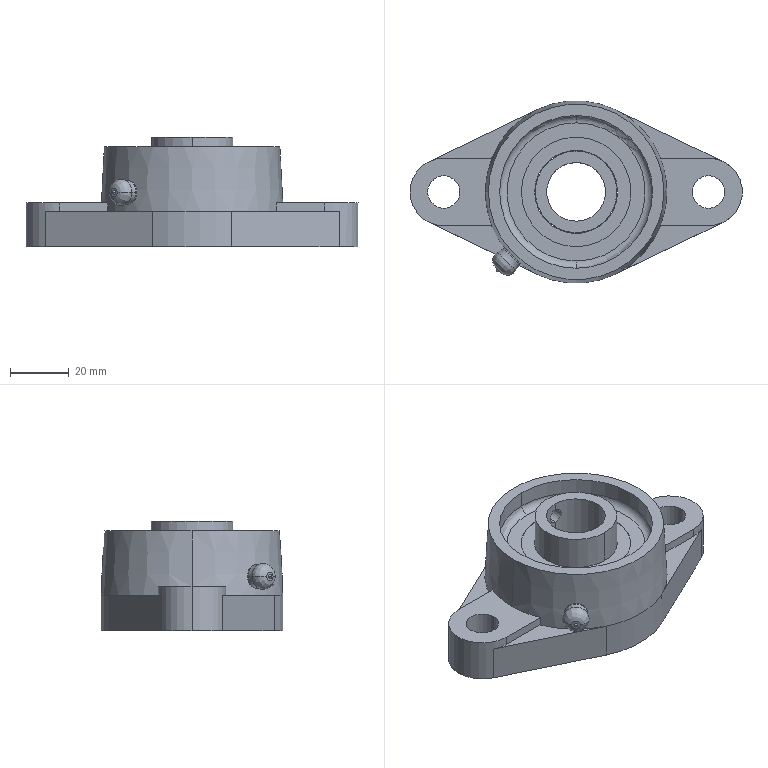Part | STEP file | 1 solid | 94 faces | box 113 x 62 x 37.3 mm | volume 69563 mm3 | cylinder 42 | plane 34 | sphere 8 | torus 6 | other 2 | cone 2 | commonest cylinder face diameters 6 x6 23 x6 37.28 x6 11 x4 28.23 x4 52 x4